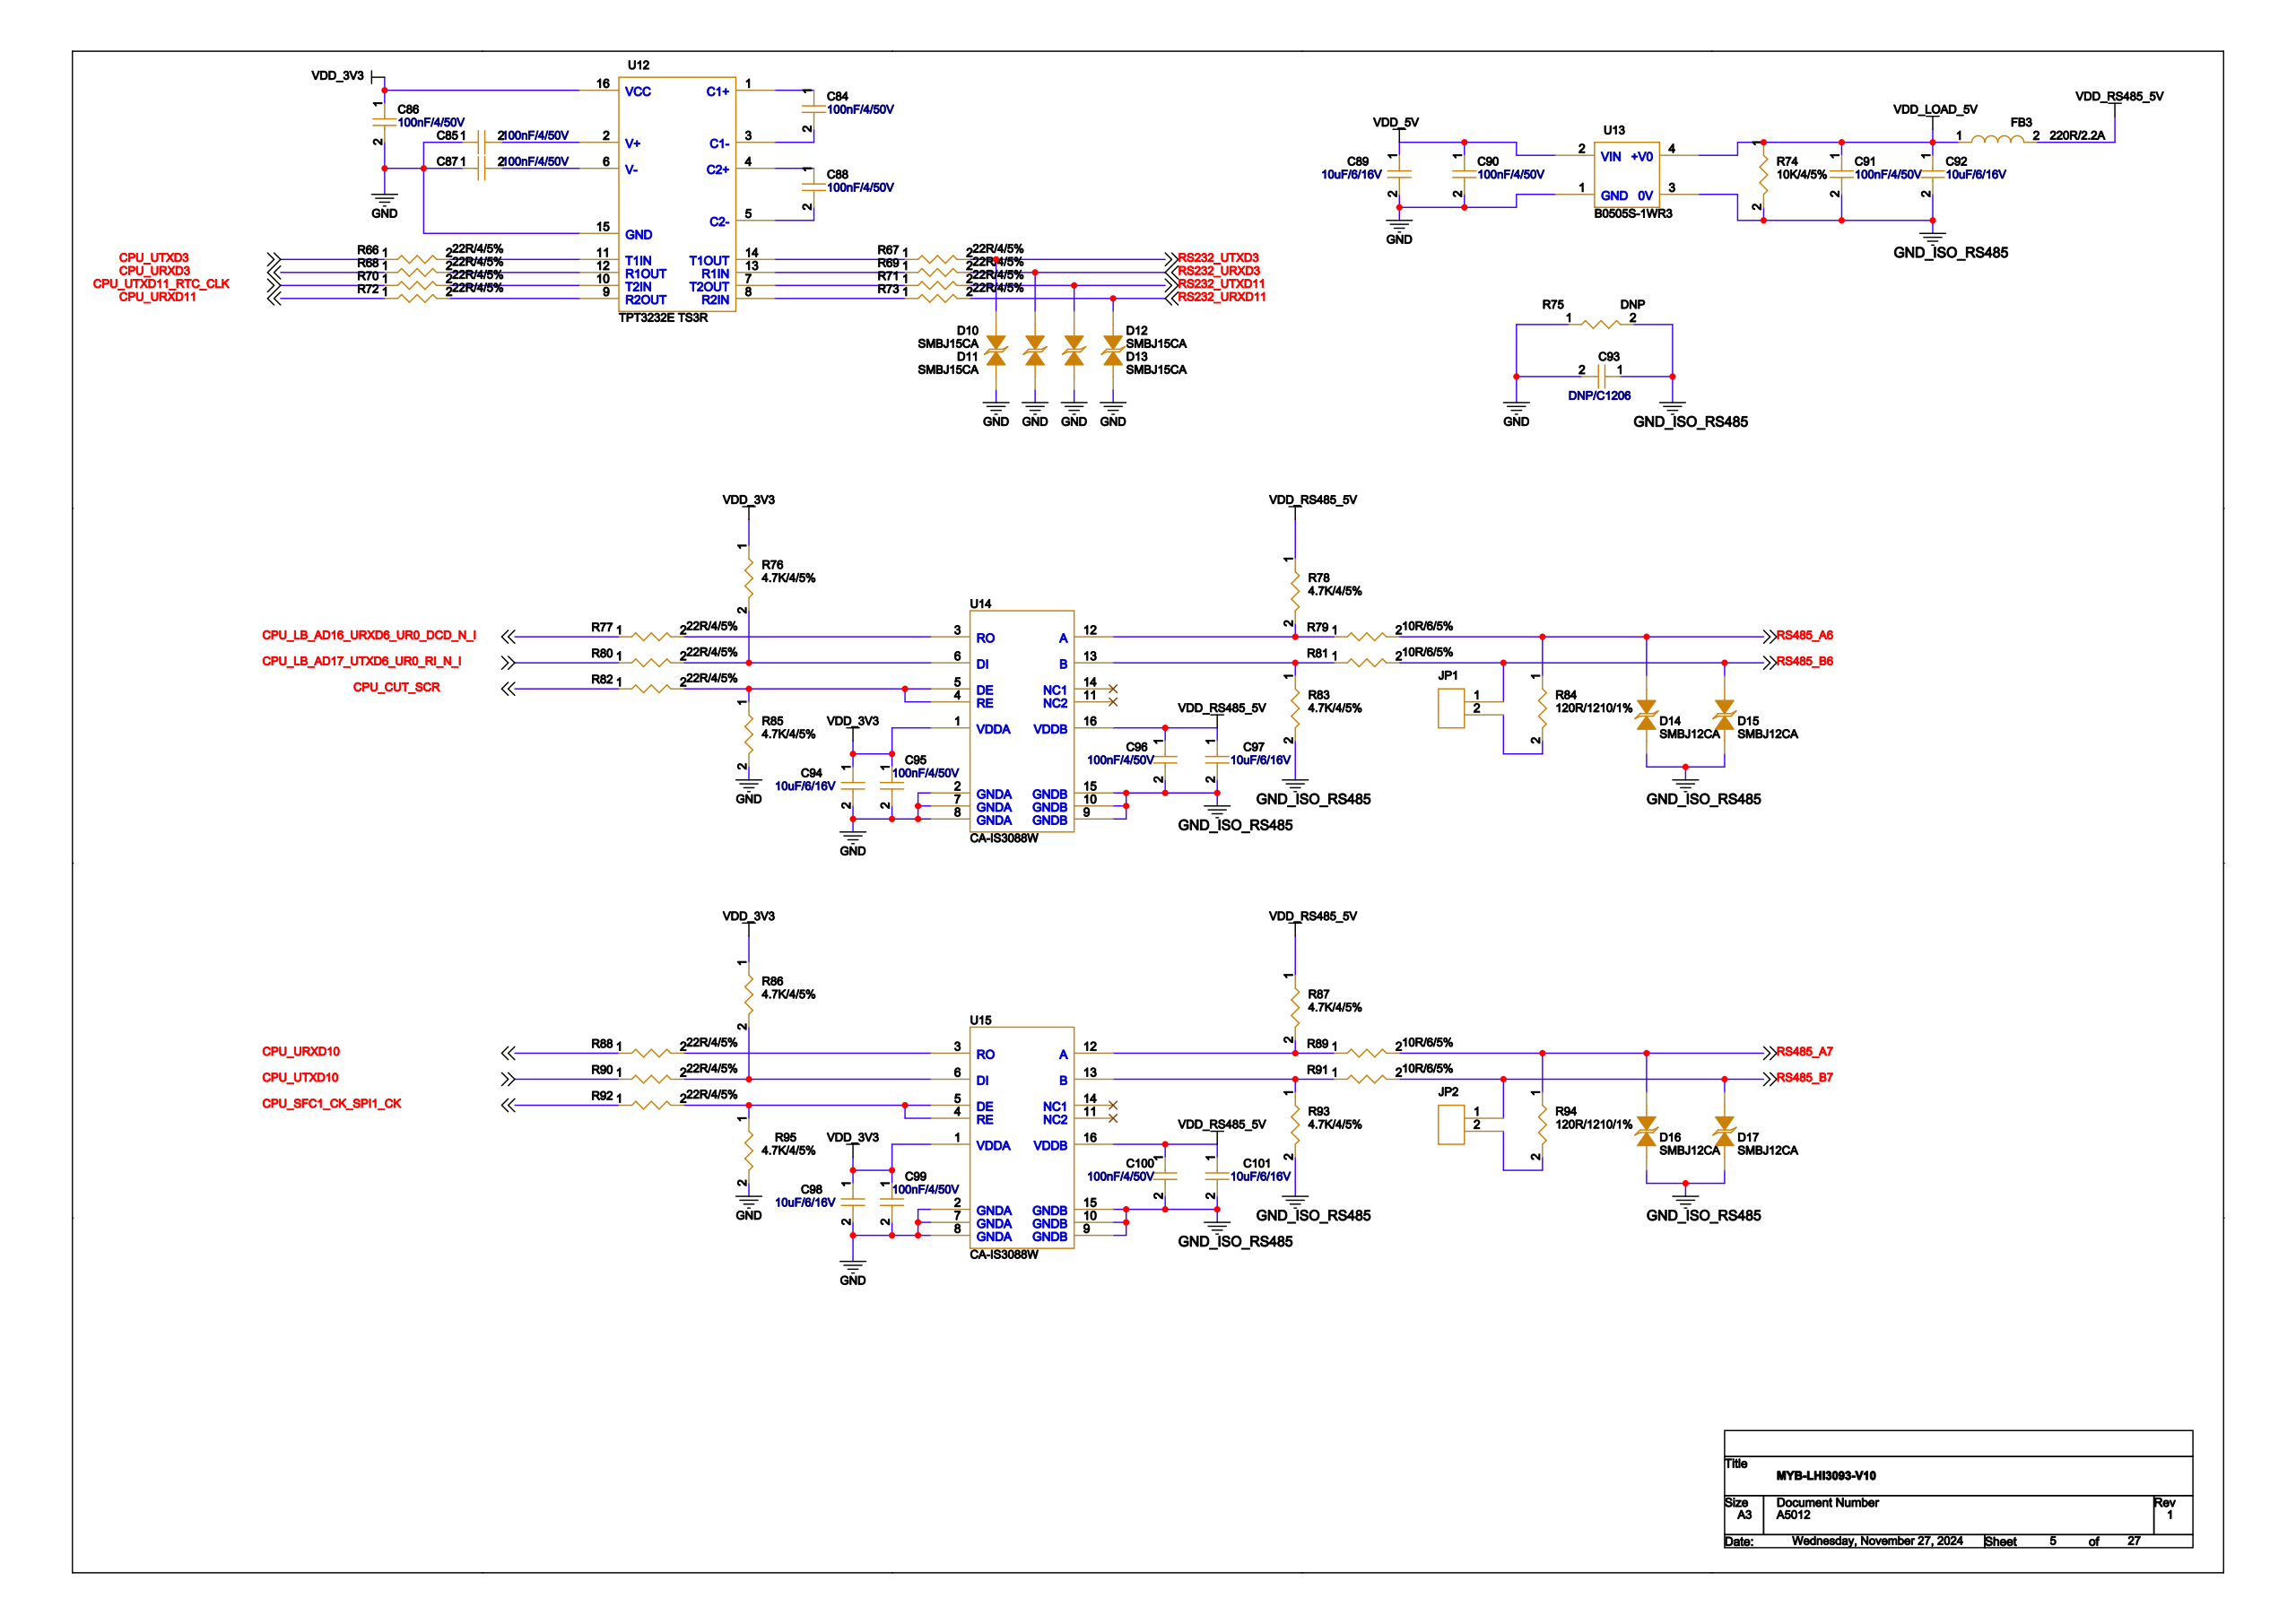Circuit board | Cadence Allegro | 1159 parts | 708 nets | one sheet of the schematic
Parts on this sheet (reference | value | footprint):
C84 | 100nF/4/50V | C0402
C85 | 100nF/4/50V | C0402
C86 | 100nF/4/50V | C0402
C87 | 100nF/4/50V | C0402
C88 | 100nF/4/50V | C0402
C89 | 10uF/6/16V | C0603
C90 | 100nF/4/50V | C0402
C91 | 100nF/4/50V | C0402
C92 | 10uF/6/16V | C0603
C93 | DNP/C1206 | C1206
C94 | 10uF/6/16V | C0603
C95 | 100nF/4/50V | C0402
C96 | 100nF/4/50V | C0402
C97 | 10uF/6/16V | C0603
C98 | 10uF/6/16V | C0603
C99 | 100nF/4/50V | C0402
C100 | 100nF/4/50V | C0402
C101 | 10uF/6/16V | C0603
D10 | SMBJ15CA | DO-214AA
D11 | SMBJ15CA | DO-214AA
D12 | SMBJ15CA | DO-214AA
D13 | SMBJ15CA | DO-214AA
D14 | SMBJ12CA | DO-214AA
D15 | SMBJ12CA | DO-214AA
D16 | SMBJ12CA | DO-214AA
D17 | SMBJ12CA | DO-214AA
FB3 | 220R/2.2A | FB0603
JP1 | CON2 | CONN1X2-2_54-DIP
JP2 | CON2 | CONN1X2-2_54-DIP
R66 | 22R/4/5% | R0402
R67 | 22R/4/5% | R0402
R68 | 22R/4/5% | R0402
R69 | 22R/4/5% | R0402
R70 | 22R/4/5% | R0402
R71 | 22R/4/5% | R0402
R72 | 22R/4/5% | R0402
R73 | 22R/4/5% | R0402
R74 | 10K/4/5% | R0402
R75 | DNP | R1206
R76 | 4.7K/4/5% | R0402
R77 | 22R/4/5% | R0402
R78 | 4.7K/4/5% | R0402
R79 | 10R/6/5% | R0603
R80 | 22R/4/5% | R0402
R81 | 10R/6/5% | R0603
R82 | 22R/4/5% | R0402
R83 | 4.7K/4/5% | R0603
R84 | 120R/1210/1% | R0603
R85 | 4.7K/4/5% | R0402
R86 | 4.7K/4/5% | R0402
R87 | 4.7K/4/5% | R0402
R88 | 22R/4/5% | R0402
R89 | 10R/6/5% | R0603
R90 | 22R/4/5% | R0402
R91 | 10R/6/5% | R0603
R92 | 22R/4/5% | R0402
R93 | 4.7K/4/5% | R0603
R94 | 120R/1210/1% | R0603
R95 | 4.7K/4/5% | R0402
U12 | TPT3232E TS3R | TSSOP16
U13 | B0505S-1WR3 | MODULE-B0505S
U14 | CA-IS3088W | SOIC16-W
U15 | CA-IS3088W | SOIC16-W
Nets of these parts (net: part-pin ...):
GND: C85-1 C86-2 C87-1 C89-2 C90-2 C93-2 C94-2 C95-2 C98-2 C99-2 D10-1 D11-1 D12-1 D13-1 R75-1 R85-2 R95-2 U12-15 U13-1 U14-2 U14-7 U14-8 U15-2 U15-7 U15-8
VDD_5V: C89-1 C90-1 U13-2
VDD_RS485_5V: C96-1 C97-1 C100-1 C101-1 FB3-2 R78-1 R87-1 U14-16 U15-16
GND_ISO_RS485: C91-2 C92-2 C93-1 C96-2 C97-2 C100-2 C101-2 D14-1 D15-1 D16-1 D17-1 R74-2 R75-2 R83-2 R93-2 U13-3 U14-9 U14-10 U14-15 U15-9 U15-10 U15-15
VDD_3V3: C86-1 C94-1 C95-1 C98-1 C99-1 R76-1 R86-1 U12-16 U14-1 U15-1
N14939273: C84-1 U12-1
N14939277: C84-2 U12-3
N14938254: C85-2 U12-2
N14938250: C87-2 U12-6
N14939284: C88-1 U12-4
N14939288: C88-2 U12-5
VDD_LOAD_5V: C91-1 C92-1 FB3-1 R74-1 U13-4
RS232_UTXD3: D10-2 R67-2
RS232_URXD3: D11-2 R69-2
RS232_UTXD11: D12-2 R71-2
RS232_URXD11: D13-2 R73-2
RS485_A6: D14-2 R79-2 R84-1
RS485_B6: D15-2 JP1-1 R81-2
RS485_A7: D16-2 R89-2 R94-1
RS485_B7: D17-2 JP2-1 R91-2
N14946133: JP1-2 R84-2
N14947831: JP2-2 R94-2
CPU_LB_AD16_URXD6_UR0_DCD_N_I: R77-1
CPU_LB_AD17_UTXD6_UR0_RI_N_I: R80-1
CPU_UTXD11_RTC_CLK: R70-1
CPU_UTXD3: R66-1
N14938442: R66-2 U12-11
N14938754: R67-1 U12-14
CPU_URXD3: R68-1
N14938446: R68-2 U12-12
N14938750: R69-1 U12-13
N14938450: R70-2 U12-10
N14938726: R71-1 U12-7
CPU_URXD11: R72-1
N14938454: R72-2 U12-9
N14938722: R73-1 U12-8
N14942394: R77-2 U14-3
N14942418: R76-2 R80-2 U14-6
CPU_CUT_SCR: R82-1
N14942573: R82-2 R85-1 U14-4 U14-5
CPU_URXD10: R88-1
N14947249: R88-2 U15-3
CPU_UTXD10: R90-1
N14947253: R86-2 R90-2 U15-6
CPU_SFC1_CK_SPI1_CK: R92-1
N14947281: R92-2 R95-1 U15-4 U15-5
N14944759: R78-2 R79-1 U14-12
N14947657: R87-2 R89-1 U15-12
N14944763: R81-1 R83-1 U14-13
N14947661: R91-1 R93-1 U15-13